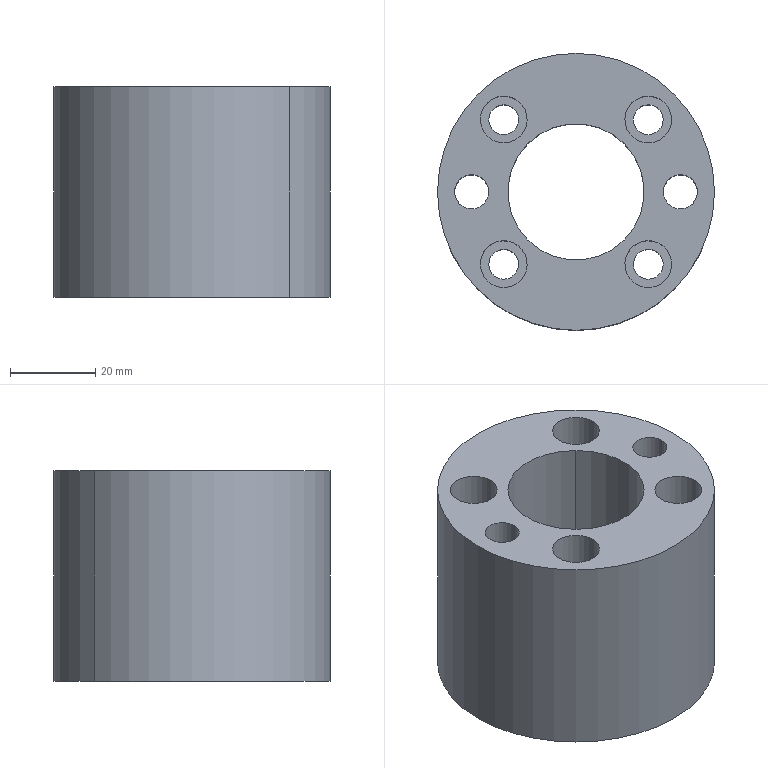Part | 1 solid | 33 faces | box 65 x 65 x 49.5 mm | volume 103481 mm3 | cylinder 26 | plane 7 | commonest cylinder face diameters 7 x8 11 x8 8 x4 32 x2 40 x2 65 x2